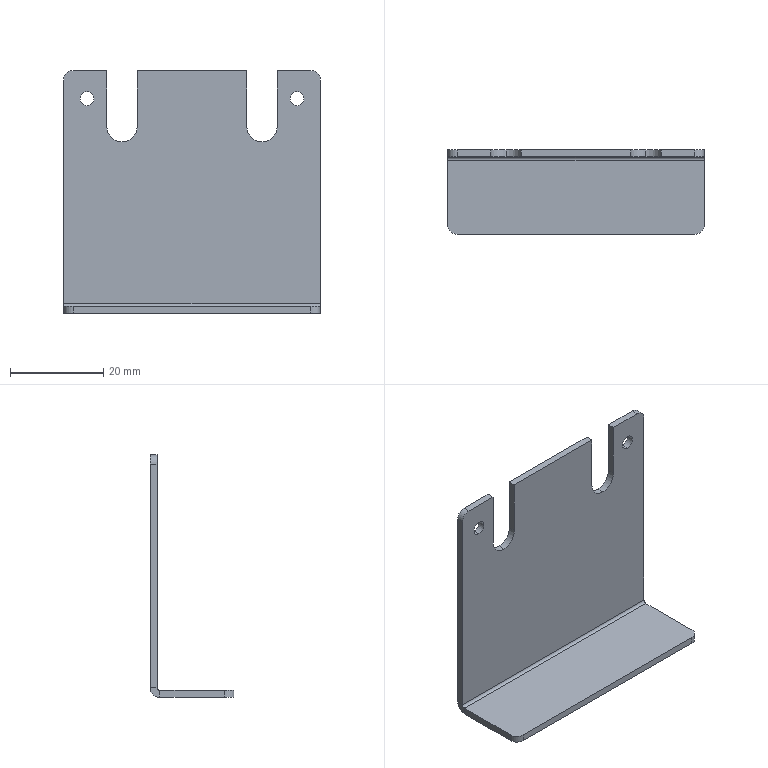Part | STEP file | 1 solid | 32 faces | box 55 x 18 x 52 mm | volume 5293 mm3 | plane 18 | cylinder 14 | commonest cylinder face diameters 3 x4 4 x4 6.5 x4 1.2 x1 4.2 x1